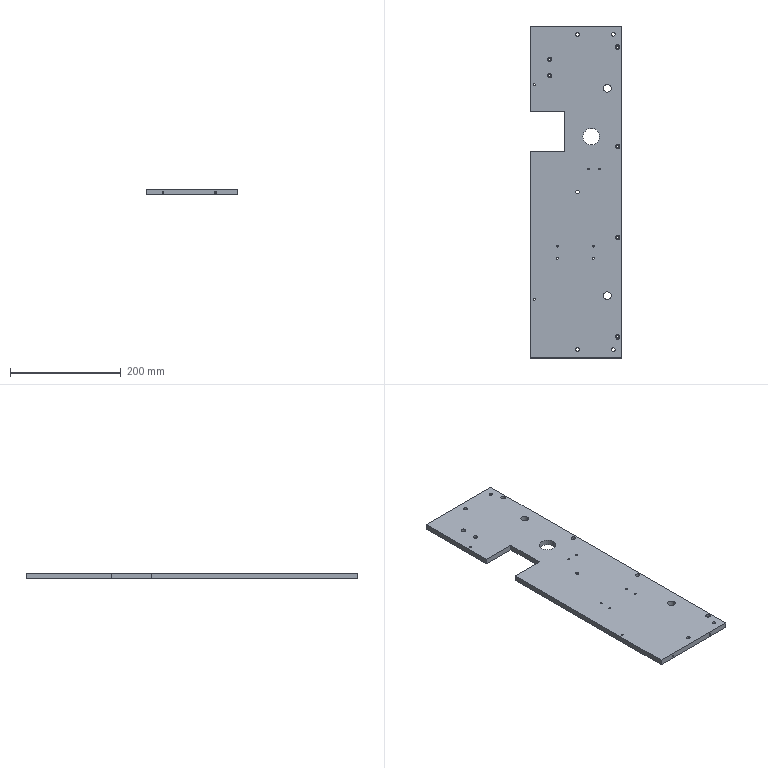Part | SolidWorks | features HoleWzd 8, Cut 2, Extrusion 1, ICE 1 | 1 solid | 103 faces | box 165 x 600 x 10 mm | volume 927945 mm3 | cylinder 74 | plane 21 | cone 8 | commonest cylinder face diameters 3.3 x20 4.5 x12 8 x12 6.6 x10 11 x10 2.5 x4